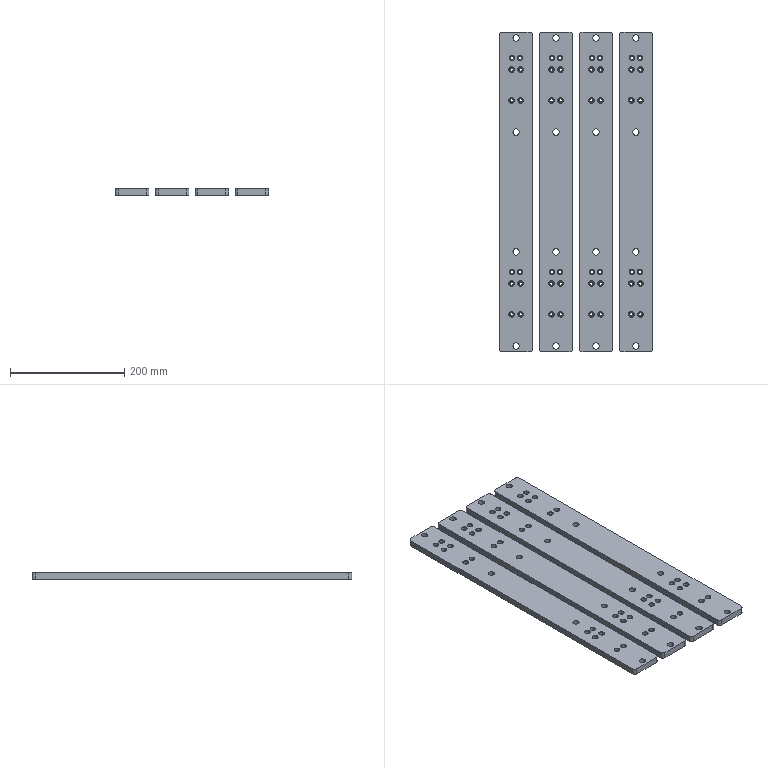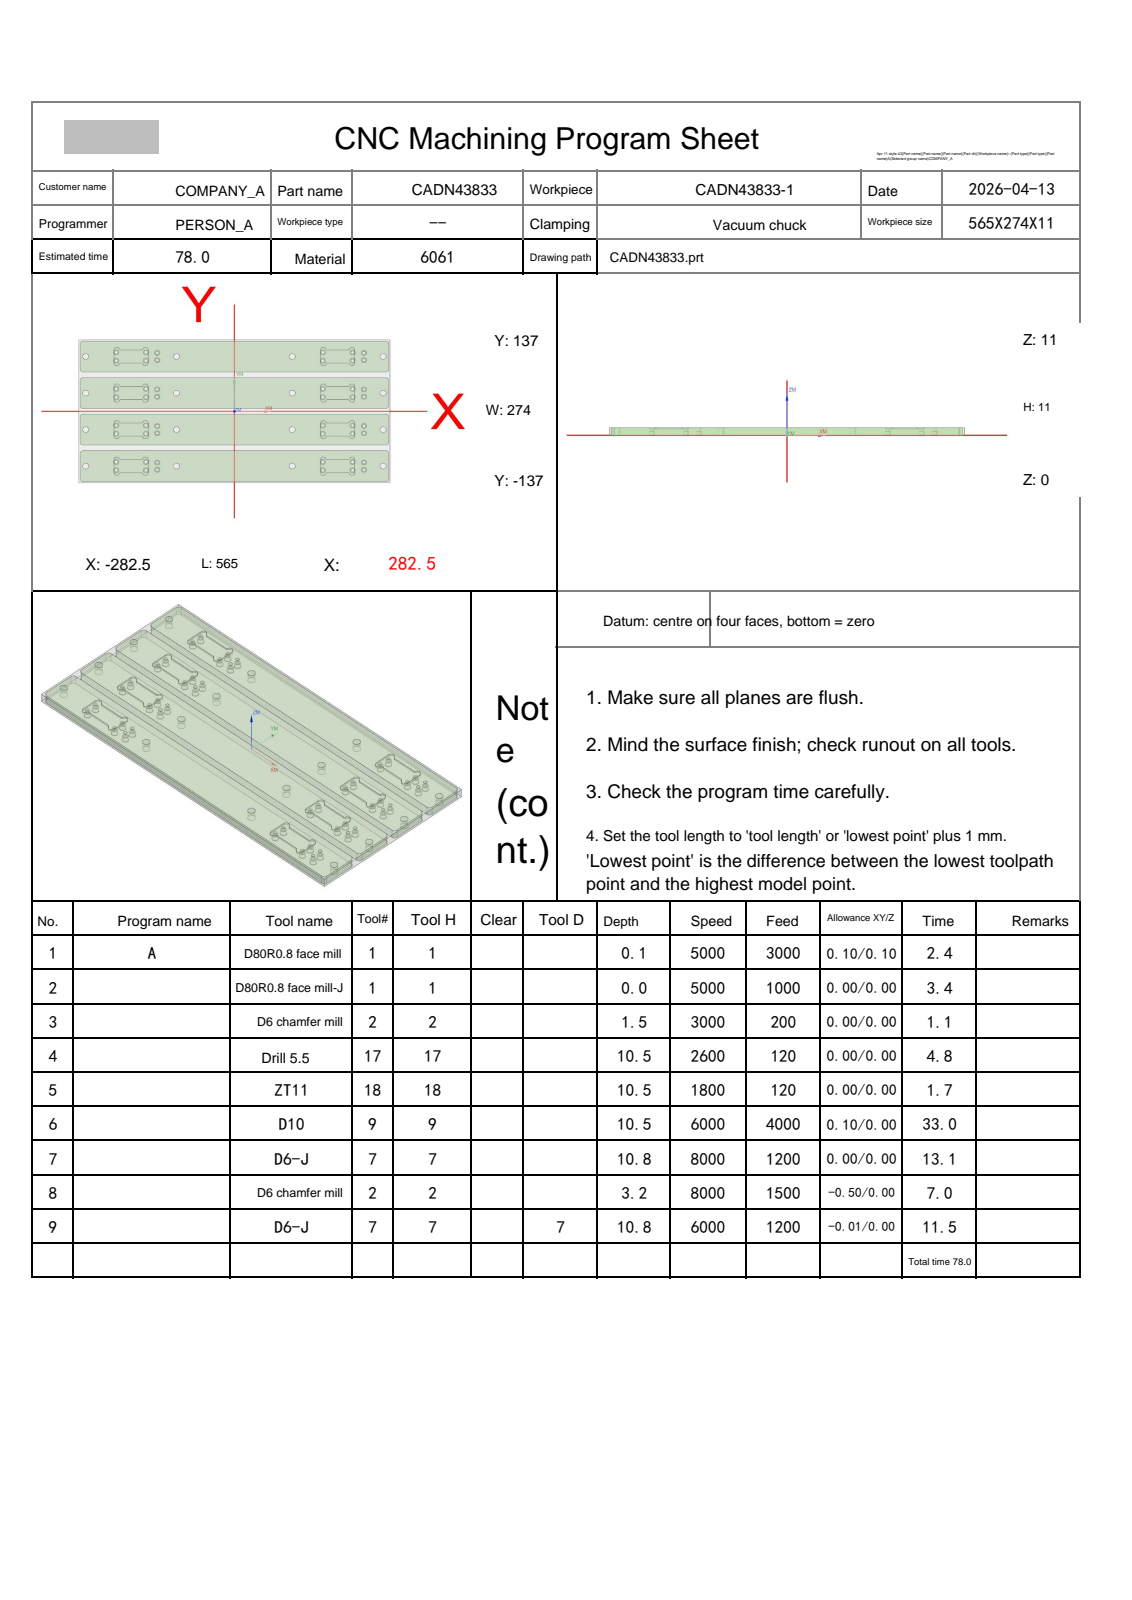NC program | NX | posted by the shop | part box 269 x 560 x 11 mm
Lines 1 to 1918 of 6644, first 1868 of 1916 lines:
%
O0001
(Machine time: 79.36 MIN)
(===Total Tool:6===)
(T1=D80R0.8 face mill D=80.  R=0.8  D-  H01 Z=11.   )
(T2=D6 chamfer mill   D=6.   R=0.   D-  H02 Z=7.8   )
(T17=drill 5.5  D=5.5  DR_a=118 D-  H17 Z=0.5   )
(T18=ZT11   D=11.  DR_a=118 D-  H18 Z=0.5   )
(T9=D10     D=10.  R=0.   D-  H09 Z=0.5   )
(T7=D6-J    D=6.   R=0.   D7  H07 Z=0.2   )
G80 G90 G17 G49 G40
G91 G28 Z0
M01
N1 T01 M06
(D80R0.8 face mill  D=80. R=0.8 H=01 ce=0.10 di=0.10)
G00 G90 G54 X-332.097 Y109.93 M03 S5000
G43 H01 Z31.
M08
Z13.55
G01 Z11.55 F3000.
X-320.097 Y110.07
X312.818 Y117.441
X312.897 Y117.442
G02 X320.097 Y110.246 I0.0 J-7.2
G01 Y80.507
Y80.493
X320.074 Y70.351
G02 X312.172 Y62.375 I-8. J.023
G01 X-312.195 Y55.103
G03 X-320.097 Y47.109 I.098 J-7.999
G01 Y10.514
Y10.486
X-320.084 Y7.204
G03 X-312.885 Y.037 I7.2 J.032
G01 X-312.805
X312.794 Y7.323
X312.873 Y7.324
G02 X320.073 Y.144 I0.0 J-7.2
G01 X320.097 Y-10.492
Y-10.508
Y-39.748
G02 X312.195 Y-47.743 I-8. J.004
G01 X-312.195 Y-55.015
G03 X-320.097 Y-63.009 I.098 J-7.999
G01 Y-102.881
G03 X-312.897 Y-110.081 I7.2 J0.0
G01 X-312.813
X320.097 Y-102.71
X332.097 Y-102.57
Z13.55
G00 X-332.097 Y109.93
Z13.1
G01 Z11.1
X-320.097 Y110.07
X312.818 Y117.441
X312.897 Y117.442
G02 X320.097 Y110.246 I0.0 J-7.2
G01 Y80.507
Y80.493
X320.074 Y70.351
G02 X312.172 Y62.375 I-8. J.023
G01 X-312.195 Y55.103
G03 X-320.097 Y47.109 I.098 J-7.999
G01 Y10.514
Y10.486
X-320.084 Y7.204
G03 X-312.885 Y.037 I7.2 J.032
G01 X-312.805
X312.794 Y7.323
X312.873 Y7.324
G02 X320.073 Y.144 I0.0 J-7.2
G01 X320.097 Y-10.492
Y-10.508
Y-39.748
G02 X312.195 Y-47.743 I-8. J.004
G01 X-312.195 Y-55.015
G03 X-320.097 Y-63.009 I.098 J-7.999
G01 Y-102.881
G03 X-312.897 Y-110.081 I7.2 J0.0
G01 X-312.813
X320.097 Y-102.71
X332.097 Y-102.57
Z13.1
G00 Z31.
G91 G28 Z0.0
M05
M09
G91 G28 Z0.0
M01
N2 T01 M06
(D80R0.8 face mill-J  D=80. R=0.8 H=01 ce=0.00 di=0.00)
G00 G90 G54 X-331.999 Y109.833 M03 S5000
G43 H01 Z31.
M08
Z13.
G01 Z11. F1000.
X-319.999 Y109.973
X312.72 Y117.35
X312.799
G02 X319.999 Y110.154 I0.0 J-7.2
G01 Y80.507
Y80.493
X319.977 Y70.307
G02 X312.075 Y62.33 I-8. J.023
G01 X-312.097 Y55.053
G03 X-319.999 Y47.059 I.098 J-7.999
G01 Y10.514
Y10.486
X-319.987 Y7.202
G03 X-312.787 Y.034 I7.2 J.032
G01 X-312.708
X312.696 Y7.326
X312.776
G02 X319.976 Y.147 I0.0 J-7.2
G01 X319.999 Y-10.493
Y-10.507
Y-39.698
G02 X312.097 Y-47.693 I-8. J.005
G01 X-312.097 Y-54.97
G03 X-319.999 Y-62.965 I.098 J-7.999
G01 Y-80.5
Y-102.794
G03 X-312.799 Y-109.989 I7.2 J.005
G01 X-312.72
X319.999 Y-102.612
X331.999 Y-102.472
Z13.
G00 Z31.
G91 G28 Z0.0
M05
M09
G91 G28 Z0.0
M01
N3 T02 M06
(D6 chamfer mill  D=6. R=0. H=02 ce=0.00 di=0.00)
G00 G90 G54 X105. Y35. M03 S3000
G43 H02 Z31.
M08
G98 G81 X105. Y35. Z9.5 R12. F200.
X160.5 Y43.
Y27.
Y-27.
Y-43.
X105. Y-35.
Y-105.
X160.5 Y-97.
Y-113.
X214.5
Y-97.
X235. Y-98.
Y-112.
X270. Y-105.
Y-35.
X235. Y-28.
Y-42.
X214.5 Y-43.
Y-27.
Y27.
Y43.
X235. Y42.
Y28.
X270. Y35.
Y105.
X235. Y112.
Y98.
X214.5 Y97.
Y113.
X160.5
Y97.
X105. Y105.
X-105.
X-140. Y112.
Y98.
X-160.5 Y97.
Y113.
X-214.5
Y97.
X-270. Y105.
Y35.
X-214.5 Y43.
Y27.
X-160.5
Y43.
X-140. Y42.
Y28.
X-105. Y35.
Y-35.
X-140. Y-42.
Y-28.
X-160.5 Y-27.
Y-43.
X-214.5
Y-27.
X-270. Y-35.
Y-105.
X-214.5 Y-97.
Y-113.
X-160.5
Y-97.
X-140. Y-98.
Y-112.
X-105. Y-105.
G80
G00 Z31.
G91 G28 Z0.0
M05
M09
G91 G28 Z0.0
M01
N4 T17 M06
(drill 5.5 D=5.5 DR_a=118 H=17)
G00 G90 G54 X-160.5 Y27. M03 S2600
G43 H17 Z31.
M08
G98 G83 X-160.5 Y27. Z.5 R12. F120. Q1.5
Y43.
X-140. Y42.
Y28.
Y-28.
X-160.5 Y-27.
Y-43.
X-140. Y-42.
Y-98.
Y-112.
X-160.5 Y-113.
Y-97.
X-214.5 Y-113.
Y-97.
Y-43.
Y-27.
Y27.
Y43.
Y97.
Y113.
X-160.5
Y97.
X-140. Y98.
Y112.
X160.5 Y113.
Y97.
Y43.
Y27.
Y-27.
Y-43.
Y-97.
Y-113.
X214.5
X235. Y-112.
Y-98.
X214.5 Y-97.
Y-43.
X235. Y-42.
Y-28.
X214.5 Y-27.
Y27.
X235. Y28.
Y42.
X214.5 Y43.
Y97.
Y113.
X235. Y112.
Y98.
G80
G00 Z31.
G91 G28 Z0.0
M05
M09
G91 G28 Z0.0
M01
N5 T18 M06
(ZT11 D=11. DR_a=118 H=18)
G00 G90 G54 X-270. Y-105. M03 S1800
G43 H18 Z31.
M08
G98 G83 X-270. Y-105. Z.5 R12. F120. Q1.5
Y-35.
Y35.
Y105.
X-105.
Y35.
Y-35.
Y-105.
X105.
Y-35.
Y35.
Y105.
X270.
Y35.
Y-35.
Y-105.
G80
G00 Z31.
G91 G28 Z0.0
M05
M09
G91 G28 Z0.0
M01
N6 T09 M06
(D10  D=10. R=0. H=09 ce=0.10 di=0.10)
G00 G90 G54 X177.82 Y-104.85 M03 S6000
G43 H09 Z31.
M08
Z11.5
M03 S6000
G01 X168.85 Z11.187 F2800.
Y-105.15 Z11.176
X187.5 Z10.525
Y-105.45
M03 S6000
X206.45 F3500.
Y-104.55
X168.55
Y-105.45
X187.5
Y-112.45
X206.792
G02 X213.45 Y-117.182 I0.0 J-7.05
G01 Y-92.818
G02 X206.792 Y-97.55 I-6.658 J2.318
G01 X168.208
G02 X161.55 Y-92.818 I0.0 J7.05
G01 Y-117.182
G02 X168.208 Y-112.45 I6.658 J-2.318
G01 X187.5
Z11.525
G00 Z12.
X177.82 Y-104.85
Z11.025
M03 S6000
G01 X168.85 Z10.712 F2800.
Y-105.15 Z10.701
X187.5 Z10.05
Y-105.45
M03 S6000
X206.45 F3500.
Y-104.55
X168.55
Y-105.45
X187.5
Y-112.45
X206.792
G02 X213.45 Y-117.182 I0.0 J-7.05
G01 Y-92.818
G02 X206.792 Y-97.55 I-6.658 J2.318
G01 X168.208
G02 X161.55 Y-92.818 I0.0 J7.05
G01 Y-117.182
G02 X168.208 Y-112.45 I6.658 J-2.318
G01 X187.5
Z11.05
G00 Z11.525
X177.82 Y-104.85
Z10.55
M03 S6000
G01 X168.85 Z10.237 F2800.
Y-105.15 Z10.226
X187.5 Z9.575
Y-105.45
M03 S6000
X206.45 F3500.
Y-104.55
X168.55
Y-105.45
X187.5
Y-112.45
X206.792
G02 X213.45 Y-117.182 I0.0 J-7.05
G01 Y-92.818
G02 X206.792 Y-97.55 I-6.658 J2.318
G01 X168.208
G02 X161.55 Y-92.818 I0.0 J7.05
G01 Y-117.182
G02 X168.208 Y-112.45 I6.658 J-2.318
G01 X187.5
Z10.575
G00 Z11.05
X177.82 Y-104.85
Z10.075
M03 S6000
G01 X168.85 Z9.762 F2800.
Y-105.15 Z9.751
X187.5 Z9.1
Y-105.45
M03 S6000
X206.45 F3500.
Y-104.55
X168.55
Y-105.45
X187.5
Y-112.45
X206.792
G02 X213.45 Y-117.182 I0.0 J-7.05
G01 Y-92.818
G02 X206.792 Y-97.55 I-6.658 J2.318
G01 X168.208
G02 X161.55 Y-92.818 I0.0 J7.05
G01 Y-117.182
G02 X168.208 Y-112.45 I6.658 J-2.318
G01 X187.5
Z10.1
G00 Z31.
X177.82 Y-34.85
Z11.5
M03 S6000
G01 X168.85 Z11.187 F2800.
Y-35.15 Z11.176
X187.5 Z10.525
Y-35.45
M03 S6000
X206.45 F3500.
Y-34.55
X168.55
Y-35.45
X187.5
Y-42.45
X206.792
G02 X213.45 Y-47.182 I0.0 J-7.05
G01 Y-22.818
G02 X206.792 Y-27.55 I-6.658 J2.318
G01 X168.208
G02 X161.55 Y-22.818 I0.0 J7.05
G01 Y-47.182
G02 X168.208 Y-42.45 I6.658 J-2.318
G01 X187.5
Z11.525
G00 Z12.
X177.82 Y-34.85
Z11.025
M03 S6000
G01 X168.85 Z10.712 F2800.
Y-35.15 Z10.701
X187.5 Z10.05
Y-35.45
M03 S6000
X206.45 F3500.
Y-34.55
X168.55
Y-35.45
X187.5
Y-42.45
X206.792
G02 X213.45 Y-47.182 I0.0 J-7.05
G01 Y-22.818
G02 X206.792 Y-27.55 I-6.658 J2.318
G01 X168.208
G02 X161.55 Y-22.818 I0.0 J7.05
G01 Y-47.182
G02 X168.208 Y-42.45 I6.658 J-2.318
G01 X187.5
Z11.05
G00 Z11.525
X177.82 Y-34.85
Z10.55
M03 S6000
G01 X168.85 Z10.237 F2800.
Y-35.15 Z10.226
X187.5 Z9.575
Y-35.45
M03 S6000
X206.45 F3500.
Y-34.55
X168.55
Y-35.45
X187.5
Y-42.45
X206.792
G02 X213.45 Y-47.182 I0.0 J-7.05
G01 Y-22.818
G02 X206.792 Y-27.55 I-6.658 J2.318
G01 X168.208
G02 X161.55 Y-22.818 I0.0 J7.05
G01 Y-47.182
G02 X168.208 Y-42.45 I6.658 J-2.318
G01 X187.5
Z10.575
G00 Z11.05
X177.82 Y-34.85
Z10.075
M03 S6000
G01 X168.85 Z9.762 F2800.
Y-35.15 Z9.751
X187.5 Z9.1
Y-35.45
M03 S6000
X206.45 F3500.
Y-34.55
X168.55
Y-35.45
X187.5
Y-42.45
X206.792
G02 X213.45 Y-47.182 I0.0 J-7.05
G01 Y-22.818
G02 X206.792 Y-27.55 I-6.658 J2.318
G01 X168.208
G02 X161.55 Y-22.818 I0.0 J7.05
G01 Y-47.182
G02 X168.208 Y-42.45 I6.658 J-2.318
G01 X187.5
Z10.1
G00 Z31.
X177.82 Y35.15
Z11.5
M03 S6000
G01 X168.85 Z11.187 F2800.
Y34.85 Z11.176
X187.5 Z10.525
Y34.55
M03 S6000
X206.45 F3500.
Y35.45
X168.55
Y34.55
X187.5
Y27.55
X206.792
G02 X213.45 Y22.818 I0.0 J-7.05
G01 Y47.182
G02 X206.792 Y42.45 I-6.658 J2.318
G01 X168.208
G02 X161.55 Y47.182 I0.0 J7.05
G01 Y22.818
G02 X168.208 Y27.55 I6.658 J-2.318
G01 X187.5
Z11.525
G00 Z12.
X177.82 Y35.15
Z11.025
M03 S6000
G01 X168.85 Z10.712 F2800.
Y34.85 Z10.701
X187.5 Z10.05
Y34.55
M03 S6000
X206.45 F3500.
Y35.45
X168.55
Y34.55
X187.5
Y27.55
X206.792
G02 X213.45 Y22.818 I0.0 J-7.05
G01 Y47.182
G02 X206.792 Y42.45 I-6.658 J2.318
G01 X168.208
G02 X161.55 Y47.182 I0.0 J7.05
G01 Y22.818
G02 X168.208 Y27.55 I6.658 J-2.318
G01 X187.5
Z11.05
G00 Z11.525
X177.82 Y35.15
Z10.55
M03 S6000
G01 X168.85 Z10.237 F2800.
Y34.85 Z10.226
X187.5 Z9.575
Y34.55
M03 S6000
X206.45 F3500.
Y35.45
X168.55
Y34.55
X187.5
Y27.55
X206.792
G02 X213.45 Y22.818 I0.0 J-7.05
G01 Y47.182
G02 X206.792 Y42.45 I-6.658 J2.318
G01 X168.208
G02 X161.55 Y47.182 I0.0 J7.05
G01 Y22.818
G02 X168.208 Y27.55 I6.658 J-2.318
G01 X187.5
Z10.575
G00 Z11.05
X177.82 Y35.15
Z10.075
M03 S6000
G01 X168.85 Z9.762 F2800.
Y34.85 Z9.751
X187.5 Z9.1
Y34.55
M03 S6000
X206.45 F3500.
Y35.45
X168.55
Y34.55
X187.5
Y27.55
X206.792
G02 X213.45 Y22.818 I0.0 J-7.05
G01 Y47.182
G02 X206.792 Y42.45 I-6.658 J2.318
G01 X168.208
G02 X161.55 Y47.182 I0.0 J7.05
G01 Y22.818
G02 X168.208 Y27.55 I6.658 J-2.318
G01 X187.5
Z10.1
G00 Z31.
X197.18 Y104.85
Z11.5
M03 S6000
G01 X206.15 Z11.187 F2800.
Y105.15 Z11.176
X187.5 Z10.525
Y105.45
M03 S6000
X168.55 F3500.
Y104.55
X206.45
Y105.45
X187.5
Y112.45
X168.208
G02 X161.55 Y117.182 I0.0 J7.05
G01 Y92.818
G02 X168.208 Y97.55 I6.658 J-2.318
G01 X206.792
G02 X213.45 Y92.818 I0.0 J-7.05
G01 Y117.182
G02 X206.792 Y112.45 I-6.658 J2.318
G01 X187.5
Z11.525
G00 Z12.
X197.18 Y104.85
Z11.025
M03 S6000
G01 X206.15 Z10.712 F2800.
Y105.15 Z10.701
X187.5 Z10.05
Y105.45
M03 S6000
X168.55 F3500.
Y104.55
X206.45
Y105.45
X187.5
Y112.45
X168.208
G02 X161.55 Y117.182 I0.0 J7.05
G01 Y92.818
G02 X168.208 Y97.55 I6.658 J-2.318
G01 X206.792
G02 X213.45 Y92.818 I0.0 J-7.05
G01 Y117.182
G02 X206.792 Y112.45 I-6.658 J2.318
G01 X187.5
Z11.05
G00 Z11.525
X197.18 Y104.85
Z10.55
M03 S6000
G01 X206.15 Z10.237 F2800.
Y105.15 Z10.226
X187.5 Z9.575
Y105.45
M03 S6000
X168.55 F3500.
Y104.55
X206.45
Y105.45
X187.5
Y112.45
X168.208
G02 X161.55 Y117.182 I0.0 J7.05
G01 Y92.818
G02 X168.208 Y97.55 I6.658 J-2.318
G01 X206.792
G02 X213.45 Y92.818 I0.0 J-7.05
G01 Y117.182
G02 X206.792 Y112.45 I-6.658 J2.318
G01 X187.5
Z10.575
G00 Z11.05
X197.18 Y104.85
Z10.075
M03 S6000
G01 X206.15 Z9.762 F2800.
Y105.15 Z9.751
X187.5 Z9.1
Y105.45
M03 S6000
X168.55 F3500.
Y104.55
X206.45
Y105.45
X187.5
Y112.45
X168.208
G02 X161.55 Y117.182 I0.0 J7.05
G01 Y92.818
G02 X168.208 Y97.55 I6.658 J-2.318
G01 X206.792
G02 X213.45 Y92.818 I0.0 J-7.05
G01 Y117.182
G02 X206.792 Y112.45 I-6.658 J2.318
G01 X187.5
Z10.1
G00 Z31.
X-177.82 Y104.85
Z11.5
M03 S6000
G01 X-168.85 Z11.187 F2800.
Y105.15 Z11.176
X-187.5 Z10.525
Y105.45
M03 S6000
X-206.45 F3500.
Y104.55
X-168.55
Y105.45
X-187.5
Y112.45
X-206.792
G02 X-213.45 Y117.182 I0.0 J7.05
G01 Y92.818
G02 X-206.792 Y97.55 I6.658 J-2.318
G01 X-168.208
G02 X-161.55 Y92.818 I0.0 J-7.05
G01 Y117.182
G02 X-168.208 Y112.45 I-6.658 J2.318
G01 X-187.5
Z11.525
G00 Z12.
X-177.82 Y104.85
Z11.025
M03 S6000
G01 X-168.85 Z10.712 F2800.
Y105.15 Z10.701
X-187.5 Z10.05
Y105.45
M03 S6000
X-206.45 F3500.
Y104.55
X-168.55
Y105.45
X-187.5
Y112.45
X-206.792
G02 X-213.45 Y117.182 I0.0 J7.05
G01 Y92.818
G02 X-206.792 Y97.55 I6.658 J-2.318
G01 X-168.208
G02 X-161.55 Y92.818 I0.0 J-7.05
G01 Y117.182
G02 X-168.208 Y112.45 I-6.658 J2.318
G01 X-187.5
Z11.05
G00 Z11.525
X-177.82 Y104.85
Z10.55
M03 S6000
G01 X-168.85 Z10.237 F2800.
Y105.15 Z10.226
X-187.5 Z9.575
Y105.45
M03 S6000
X-206.45 F3500.
Y104.55
X-168.55
Y105.45
X-187.5
Y112.45
X-206.792
G02 X-213.45 Y117.182 I0.0 J7.05
G01 Y92.818
G02 X-206.792 Y97.55 I6.658 J-2.318
G01 X-168.208
G02 X-161.55 Y92.818 I0.0 J-7.05
G01 Y117.182
G02 X-168.208 Y112.45 I-6.658 J2.318
G01 X-187.5
Z10.575
G00 Z11.05
X-177.82 Y104.85
Z10.075
M03 S6000
G01 X-168.85 Z9.762 F2800.
Y105.15 Z9.751
X-187.5 Z9.1
Y105.45
M03 S6000
X-206.45 F3500.
Y104.55
X-168.55
Y105.45
X-187.5
Y112.45
X-206.792
G02 X-213.45 Y117.182 I0.0 J7.05
G01 Y92.818
G02 X-206.792 Y97.55 I6.658 J-2.318
G01 X-168.208
G02 X-161.55 Y92.818 I0.0 J-7.05
G01 Y117.182
G02 X-161.664 Y116.878 I-6.658 J2.318
X-168.208 Y112.45 I-6.544 J2.622
G01 X-187.5
Z10.1
G00 Z31.
X-177.82 Y34.85
Z11.5
M03 S6000
G01 X-168.85 Z11.187 F2800.
Y35.15 Z11.176
X-187.5 Z10.525
Y35.45
M03 S6000
X-206.45 F3500.
Y34.55
X-168.55
Y35.45
X-187.5
Y42.45
X-206.792
G02 X-213.45 Y47.182 I0.0 J7.05
G01 Y22.818
G02 X-206.792 Y27.55 I6.658 J-2.318
G01 X-168.208
G02 X-161.56 Y22.847 I0.0 J-7.05
G01 X-161.55 Y22.836
Y47.166
X-161.56 Y47.153
G02 X-168.208 Y42.45 I-6.648 J2.347
G01 X-187.5
Z11.525
G00 Z12.
X-177.82 Y34.85
Z11.025
M03 S6000
G01 X-168.85 Z10.712 F2800.
Y35.15 Z10.701
X-187.5 Z10.05
Y35.45
M03 S6000
X-206.45 F3500.
Y34.55
X-168.55
Y35.45
X-187.5
Y42.45
X-206.792
G02 X-213.45 Y47.182 I0.0 J7.05
G01 Y22.818
G02 X-206.792 Y27.55 I6.658 J-2.318
G01 X-168.208
G02 X-161.56 Y22.847 I0.0 J-7.05
G01 X-161.55 Y22.836
Y47.166
X-161.56 Y47.153
G02 X-168.208 Y42.45 I-6.648 J2.347
G01 X-187.5
Z11.05
G00 Z11.525
X-177.82 Y34.85
Z10.55
M03 S6000
G01 X-168.85 Z10.237 F2800.
Y35.15 Z10.226
X-187.5 Z9.575
Y35.45
M03 S6000
X-206.45 F3500.
Y34.55
X-168.55
Y35.45
X-187.5
Y42.45
X-206.792
G02 X-213.45 Y47.182 I0.0 J7.05
G01 Y22.818
G02 X-206.792 Y27.55 I6.658 J-2.318
G01 X-168.208
G02 X-161.56 Y22.847 I0.0 J-7.05
G01 X-161.55 Y22.836
Y47.166
X-161.56 Y47.153
G02 X-168.208 Y42.45 I-6.648 J2.347
G01 X-187.5
Z10.575
G00 Z11.05
X-177.82 Y34.85
Z10.075
M03 S6000
G01 X-168.85 Z9.762 F2800.
Y35.15 Z9.751
X-187.5 Z9.1
Y35.45
M03 S6000
X-206.45 F3500.
Y34.55
X-168.55
Y35.45
X-187.5
Y42.45
X-206.792
G02 X-213.45 Y47.182 I0.0 J7.05
G01 Y22.818
G02 X-206.792 Y27.55 I6.658 J-2.318
G01 X-168.208
G02 X-161.56 Y22.847 I0.0 J-7.05
G01 X-161.55 Y22.836
Y47.166
X-161.56 Y47.153
G02 X-168.208 Y42.45 I-6.648 J2.347
G01 X-187.5
Z10.1
G00 Z31.
X-177.82 Y-35.15
Z11.5
M03 S6000
G01 X-168.85 Z11.187 F2800.
Y-34.85 Z11.176
X-187.5 Z10.525
Y-34.55
M03 S6000
X-206.45 F3500.
Y-35.45
X-168.55
Y-34.55
X-187.5
Y-27.55
X-206.792
G02 X-213.45 Y-22.818 I0.0 J7.05
G01 Y-47.182
G02 X-206.792 Y-42.45 I6.658 J-2.318
G01 X-168.208
G02 X-161.55 Y-47.182 I0.0 J-7.05
G01 Y-22.818
G02 X-168.208 Y-27.55 I-6.658 J2.318
G01 X-187.5
Z11.525
G00 Z12.
X-177.82 Y-35.15
Z11.025
M03 S6000
G01 X-168.85 Z10.712 F2800.
Y-34.85 Z10.701
X-187.5 Z10.05
Y-34.55
M03 S6000
X-206.45 F3500.
Y-35.45
X-168.55
Y-34.55
X-187.5
Y-27.55
X-206.792
G02 X-213.45 Y-22.818 I0.0 J7.05
G01 Y-47.182
G02 X-206.792 Y-42.45 I6.658 J-2.318
G01 X-168.208
G02 X-161.55 Y-47.182 I0.0 J-7.05
G01 Y-22.818
G02 X-168.208 Y-27.55 I-6.658 J2.318
G01 X-187.5
Z11.05
G00 Z11.525
X-177.82 Y-35.15
Z10.55
M03 S6000
G01 X-168.85 Z10.237 F2800.
Y-34.85 Z10.226
X-187.5 Z9.575
Y-34.55
M03 S6000
X-206.45 F3500.
Y-35.45
X-168.55
Y-34.55
X-187.5
Y-27.55
X-206.792
G02 X-213.45 Y-22.818 I0.0 J7.05
G01 Y-47.144
Y-47.182
G02 X-206.792 Y-42.45 I6.658 J-2.318
G01 X-168.208
G02 X-161.55 Y-47.182 I0.0 J-7.05
G01 Y-22.818
G02 X-168.208 Y-27.55 I-6.658 J2.318
G01 X-187.5
Z10.575
G00 Z11.05
X-177.82 Y-35.15
Z10.075
M03 S6000
G01 X-168.85 Z9.762 F2800.
Y-34.85 Z9.751
X-187.5 Z9.1
Y-34.55
M03 S6000
X-206.45 F3500.
Y-35.45
X-168.55
Y-34.55
X-187.5
Y-27.55
X-206.792
G02 X-213.45 Y-22.818 I0.0 J7.05
G01 Y-47.144
Y-47.182
G02 X-206.792 Y-42.45 I6.658 J-2.318
G01 X-168.208
G02 X-161.55 Y-47.182 I0.0 J-7.05
G01 Y-22.818
G02 X-168.208 Y-27.55 I-6.658 J2.318
G01 X-187.5
Z10.1
G00 Z31.
X-197.18 Y-104.85
Z11.5
M03 S6000
G01 X-206.15 Z11.187 F2800.
Y-105.15 Z11.176
X-187.5 Z10.525
Y-105.45
M03 S6000
X-168.55 F3500.
Y-104.55
X-206.45
Y-105.45
X-187.5
Y-112.45
X-168.208
G02 X-161.55 Y-117.182 I0.0 J-7.05
G01 Y-92.818
G02 X-168.208 Y-97.55 I-6.658 J2.318
G01 X-206.792
G02 X-213.45 Y-92.818 I0.0 J7.05
G01 Y-117.182
G02 X-206.792 Y-112.45 I6.658 J-2.318
G01 X-187.5
Z11.525
G00 Z12.
X-197.18 Y-104.85
Z11.025
M03 S6000
G01 X-206.15 Z10.712 F2800.
Y-105.15 Z10.701
X-187.5 Z10.05
Y-105.45
M03 S6000
X-168.55 F3500.
Y-104.55
X-206.45
Y-105.45
X-187.5
Y-112.45
X-168.208
G02 X-161.55 Y-117.182 I0.0 J-7.05
G01 Y-92.818
G02 X-168.208 Y-97.55 I-6.658 J2.318
G01 X-206.792
G02 X-213.45 Y-92.818 I0.0 J7.05
G01 Y-117.182
G02 X-206.792 Y-112.45 I6.658 J-2.318
G01 X-187.5
Z11.05
G00 Z11.525
X-197.18 Y-104.85
Z10.55
M03 S6000
G01 X-206.15 Z10.237 F2800.
Y-105.15 Z10.226
X-187.5 Z9.575
Y-105.45
M03 S6000
X-168.55 F3500.
Y-104.55
X-206.45
Y-105.45
X-187.5
Y-112.45
X-168.208
G02 X-161.55 Y-117.182 I0.0 J-7.05
G01 Y-92.818
G02 X-161.654 Y-93.098 I-6.658 J2.318
X-168.208 Y-97.55 I-6.554 J2.598
G01 X-206.792
G02 X-213.45 Y-92.818 I0.0 J7.05
G01 Y-117.182
G02 X-206.792 Y-112.45 I6.658 J-2.318
G01 X-187.5
Z10.575
G00 Z11.05
X-197.18 Y-104.85
Z10.075
M03 S6000
G01 X-206.15 Z9.762 F2800.
Y-105.15 Z9.751
X-187.5 Z9.1
Y-105.45
M03 S6000
X-168.55 F3500.
Y-104.55
X-206.45
Y-105.45
X-187.5
Y-112.45
X-168.208
G02 X-161.55 Y-117.182 I0.0 J-7.05
G01 Y-92.818
X-161.568 Y-92.869
G02 X-168.208 Y-97.55 I-6.64 J2.369
G01 X-206.792
G02 X-213.45 Y-92.818 I0.0 J7.05
G01 Y-117.182
G02 X-206.792 Y-112.45 I6.658 J-2.318
G01 X-187.5
Z10.1
G00 Z31.
G00 G90 X0.0 Y139.6 M03 S6000
Z31.
Z11.5
G01 X275. Z11.396 F4000.
G02 X285.1 Y129.5 Z11.39 I0.0 J-10.1
G01 Y80.5 Z11.371
G02 X275. Y70.4 Z11.365 I-10.1 J0.0
G01 X-275. Z11.157
G02 X-285.1 Y80.5 Z11.151 I0.0 J10.1
G01 Y129.5 Z11.132
G02 X-275. Y139.6 Z11.126 I10.1 J0.0
G01 X275. Z10.917
G02 X285.1 Y129.5 Z10.911 I0.0 J-10.1
G01 Y80.5 Z10.893
G02 X275. Y70.4 Z10.887 I-10.1 J0.0
G01 X-275. Z10.678
G02 X-285.1 Y80.5 Z10.672 I0.0 J10.1
G01 Y129.5 Z10.654
G02 X-275. Y139.6 Z10.648 I10.1 J0.0
G01 X275. Z10.439
G02 X285.1 Y129.5 Z10.433 I0.0 J-10.1
G01 Y80.5 Z10.415
G02 X275. Y70.4 Z10.409 I-10.1 J0.0
G01 X-275. Z10.2
G02 X-285.1 Y80.5 Z10.194 I0.0 J10.1
G01 Y129.5 Z10.175
G02 X-275. Y139.6 Z10.169 I10.1 J0.0
G01 X275. Z9.961
G02 X285.1 Y129.5 Z9.955 I0.0 J-10.1
G01 Y80.5 Z9.936
G02 X275. Y70.4 Z9.93 I-10.1 J0.0
G01 X-275. Z9.722
G02 X-285.1 Y80.5 Z9.716 I0.0 J10.1
G01 Y129.5 Z9.697
G02 X-275. Y139.6 Z9.691 I10.1 J0.0
G01 X275. Z9.483
G02 X285.1 Y129.5 Z9.477 I0.0 J-10.1
G01 Y80.5 Z9.458
G02 X275. Y70.4 Z9.452 I-10.1 J0.0
G01 X-275. Z9.244
G02 X-285.1 Y80.5 Z9.238 I0.0 J10.1
G01 Y129.5 Z9.219
G02 X-275. Y139.6 Z9.213 I10.1 J0.0
G01 X275. Z9.004
G02 X285.1 Y129.5 Z8.998 I0.0 J-10.1
G01 Y80.5 Z8.98
G02 X275. Y70.4 Z8.974 I-10.1 J0.0
G01 X-275. Z8.765
G02 X-285.1 Y80.5 Z8.759 I0.0 J10.1
G01 Y129.5 Z8.741
G02 X-275. Y139.6 Z8.735 I10.1 J0.0
G01 X275. Z8.526
G02 X285.1 Y129.5 Z8.52 I0.0 J-10.1
G01 Y80.5 Z8.502
G02 X275. Y70.4 Z8.496 I-10.1 J0.0
G01 X-275. Z8.287
G02 X-285.1 Y80.5 Z8.281 I0.0 J10.1
G01 Y129.5 Z8.262
G02 X-275. Y139.6 Z8.256 I10.1 J0.0
G01 X275. Z8.048
G02 X285.1 Y129.5 Z8.042 I0.0 J-10.1
G01 Y80.5 Z8.023
G02 X275. Y70.4 Z8.017 I-10.1 J0.0
G01 X-275. Z7.809
G02 X-285.1 Y80.5 Z7.803 I0.0 J10.1
G01 Y129.5 Z7.784
G02 X-275. Y139.6 Z7.778 I10.1 J0.0
G01 X275. Z7.57
G02 X285.1 Y129.5 Z7.564 I0.0 J-10.1
G01 Y80.5 Z7.545
G02 X275. Y70.4 Z7.539 I-10.1 J0.0
G01 X-275. Z7.331
G02 X-285.1 Y80.5 Z7.325 I0.0 J10.1
G01 Y129.5 Z7.306
G02 X-275. Y139.6 Z7.3 I10.1 J0.0
G01 X275. Z7.091
G02 X285.1 Y129.5 Z7.085 I0.0 J-10.1
G01 Y80.5 Z7.067
G02 X275. Y70.4 Z7.061 I-10.1 J0.0
G01 X-275. Z6.852
G02 X-285.1 Y80.5 Z6.846 I0.0 J10.1
G01 Y129.5 Z6.828
G02 X-275. Y139.6 Z6.822 I10.1 J0.0
G01 X275. Z6.613
G02 X285.1 Y129.5 Z6.607 I0.0 J-10.1
G01 Y80.5 Z6.589
G02 X275. Y70.4 Z6.583 I-10.1 J0.0
G01 X-275. Z6.374
G02 X-285.1 Y80.5 Z6.368 I0.0 J10.1
G01 Y129.5 Z6.349
G02 X-275. Y139.6 Z6.343 I10.1 J0.0
G01 X275. Z6.135
G02 X285.1 Y129.5 Z6.129 I0.0 J-10.1
G01 Y80.5 Z6.11
G02 X275. Y70.4 Z6.104 I-10.1 J0.0
G01 X-275. Z5.896
G02 X-285.1 Y80.5 Z5.89 I0.0 J10.1
G01 Y129.5 Z5.871
G02 X-275. Y139.6 Z5.865 I10.1 J0.0
G01 X275. Z5.657
G02 X285.1 Y129.5 Z5.651 I0.0 J-10.1
G01 Y80.5 Z5.632
G02 X275. Y70.4 Z5.626 I-10.1 J0.0
G01 X-275. Z5.417
G02 X-285.1 Y80.5 Z5.411 I0.0 J10.1
G01 Y129.5 Z5.393
G02 X-275. Y139.6 Z5.387 I10.1 J0.0
G01 X275. Z5.178
G02 X285.1 Y129.5 Z5.172 I0.0 J-10.1
G01 Y80.5 Z5.154
G02 X275. Y70.4 Z5.148 I-10.1 J0.0
G01 X-275. Z4.939
G02 X-285.1 Y80.5 Z4.933 I0.0 J10.1
G01 Y129.5 Z4.915
G02 X-275. Y139.6 Z4.909 I10.1 J0.0
G01 X275. Z4.7
G02 X285.1 Y129.5 Z4.694 I0.0 J-10.1
G01 Y80.5 Z4.675
G02 X275. Y70.4 Z4.669 I-10.1 J0.0
G01 X-275. Z4.461
G02 X-285.1 Y80.5 Z4.455 I0.0 J10.1
G01 Y129.5 Z4.436
G02 X-275. Y139.6 Z4.43 I10.1 J0.0
G01 X275. Z4.222
G02 X285.1 Y129.5 Z4.216 I0.0 J-10.1
G01 Y80.5 Z4.197
G02 X275. Y70.4 Z4.191 I-10.1 J0.0
G01 X-275. Z3.983
G02 X-285.1 Y80.5 Z3.977 I0.0 J10.1
G01 Y129.5 Z3.958
G02 X-275. Y139.6 Z3.952 I10.1 J0.0
G01 X275. Z3.744
G02 X285.1 Y129.5 Z3.738 I0.0 J-10.1
G01 Y80.5 Z3.719
G02 X275. Y70.4 Z3.713 I-10.1 J0.0
G01 X-275. Z3.504
G02 X-285.1 Y80.5 Z3.498 I0.0 J10.1
G01 Y129.5 Z3.48
G02 X-275. Y139.6 Z3.474 I10.1 J0.0
G01 X275. Z3.265
G02 X285.1 Y129.5 Z3.259 I0.0 J-10.1
G01 Y80.5 Z3.241
G02 X275. Y70.4 Z3.235 I-10.1 J0.0
G01 X-275. Z3.026
G02 X-285.1 Y80.5 Z3.02 I0.0 J10.1
G01 Y129.5 Z3.002
G02 X-275. Y139.6 Z2.996 I10.1 J0.0
G01 X275. Z2.787
G02 X285.1 Y129.5 Z2.781 I0.0 J-10.1
G01 Y80.5 Z2.762
G02 X275. Y70.4 Z2.756 I-10.1 J0.0
G01 X-275. Z2.548
G02 X-285.1 Y80.5 Z2.542 I0.0 J10.1
G01 Y129.5 Z2.523
G02 X-275. Y139.6 Z2.517 I10.1 J0.0
G01 X275. Z2.309
G02 X285.1 Y129.5 Z2.303 I0.0 J-10.1
G01 Y80.5 Z2.284
G02 X275. Y70.4 Z2.278 I-10.1 J0.0
G01 X-275. Z2.07
G02 X-285.1 Y80.5 Z2.064 I0.0 J10.1
G01 Y129.5 Z2.045
G02 X-275. Y139.6 Z2.039 I10.1 J0.0
G01 X275. Z1.831
G02 X285.1 Y129.5 Z1.825 I0.0 J-10.1
G01 Y80.5 Z1.806
G02 X275. Y70.4 Z1.8 I-10.1 J0.0
G01 X-275. Z1.591
G02 X-285.1 Y80.5 Z1.585 I0.0 J10.1
G01 Y129.5 Z1.567
G02 X-275. Y139.6 Z1.561 I10.1 J0.0
G01 X275. Z1.352
G02 X285.1 Y129.5 Z1.346 I0.0 J-10.1
G01 Y80.5 Z1.328
G02 X275. Y70.4 Z1.322 I-10.1 J0.0
G01 X-275. Z1.113
G02 X-285.1 Y80.5 Z1.107 I0.0 J10.1
G01 Y129.5 Z1.089
G02 X-275. Y139.6 Z1.083 I10.1 J0.0
G01 X275. Z.874
G02 X285.1 Y129.5 Z.868 I0.0 J-10.1
G01 Y80.5 Z.849
G02 X275. Y70.4 Z.843 I-10.1 J0.0
G01 X-275. Z.635
G02 X-285.1 Y80.5 Z.629 I0.0 J10.1
G01 Y129.5 Z.61
G02 X-275. Y139.6 Z.604 I10.1 J0.0
G01 X0.0 Z.5
X275.
G02 X285.1 Y129.5 I0.0 J-10.1
G01 Y80.5
G02 X275. Y70.4 I-10.1 J0.0
G01 X-275.
G02 X-285.1 Y80.5 I0.0 J10.1
G01 Y129.5
G02 X-275. Y139.6 I10.1 J0.0
G01 X0.0
X.5
Z1.5
G00 Z31.
X0.0 Y69.6
Z11.5
G01 X275. Z11.396
G02 X285.1 Y59.5 Z11.39 I0.0 J-10.1
G01 Y10.5 Z11.371
G02 X275. Y.4 Z11.365 I-10.1 J0.0
G01 X-275. Z11.157
G02 X-285.1 Y10.5 Z11.151 I0.0 J10.1
G01 Y59.5 Z11.132
G02 X-275. Y69.6 Z11.126 I10.1 J0.0
G01 X275. Z10.917
G02 X285.1 Y59.5 Z10.911 I0.0 J-10.1
G01 Y10.5 Z10.893
G02 X275. Y.4 Z10.887 I-10.1 J0.0
G01 X-275. Z10.678
G02 X-285.1 Y10.5 Z10.672 I0.0 J10.1
G01 Y59.5 Z10.654
G02 X-275. Y69.6 Z10.648 I10.1 J0.0
G01 X275. Z10.439
G02 X285.1 Y59.5 Z10.433 I0.0 J-10.1
G01 Y10.5 Z10.415
G02 X275. Y.4 Z10.409 I-10.1 J0.0
G01 X-275. Z10.2
G02 X-285.1 Y10.5 Z10.194 I0.0 J10.1
G01 Y59.5 Z10.175
G02 X-275. Y69.6 Z10.169 I10.1 J0.0
G01 X275. Z9.961
G02 X285.1 Y59.5 Z9.955 I0.0 J-10.1
G01 Y10.5 Z9.936
G02 X275. Y.4 Z9.93 I-10.1 J0.0
G01 X-275. Z9.722
G02 X-285.1 Y10.5 Z9.716 I0.0 J10.1
G01 Y59.5 Z9.697
G02 X-275. Y69.6 Z9.691 I10.1 J0.0
G01 X275. Z9.483
G02 X285.1 Y59.5 Z9.477 I0.0 J-10.1
G01 Y10.5 Z9.458
G02 X275. Y.4 Z9.452 I-10.1 J0.0
G01 X-275. Z9.244
G02 X-285.1 Y10.5 Z9.238 I0.0 J10.1
G01 Y59.5 Z9.219
G02 X-275. Y69.6 Z9.213 I10.1 J0.0
G01 X275. Z9.004
G02 X285.1 Y59.5 Z8.998 I0.0 J-10.1
G01 Y10.5 Z8.98
G02 X275. Y.4 Z8.974 I-10.1 J0.0
G01 X-275. Z8.765
G02 X-285.1 Y10.5 Z8.759 I0.0 J10.1
G01 Y59.5 Z8.741
G02 X-275. Y69.6 Z8.735 I10.1 J0.0
G01 X275. Z8.526
G02 X285.1 Y59.5 Z8.52 I0.0 J-10.1
G01 Y10.5 Z8.502
G02 X275. Y.4 Z8.496 I-10.1 J0.0
G01 X-275. Z8.287
G02 X-285.1 Y10.5 Z8.281 I0.0 J10.1
G01 Y59.5 Z8.262
G02 X-275. Y69.6 Z8.256 I10.1 J0.0
G01 X275. Z8.048
G02 X285.1 Y59.5 Z8.042 I0.0 J-10.1
G01 Y10.5 Z8.023
G02 X275. Y.4 Z8.017 I-10.1 J0.0
G01 X-275. Z7.809
G02 X-285.1 Y10.5 Z7.803 I0.0 J10.1
G01 Y59.5 Z7.784
G02 X-275. Y69.6 Z7.778 I10.1 J0.0
G01 X275. Z7.57
G02 X285.1 Y59.5 Z7.564 I0.0 J-10.1
G01 Y10.5 Z7.545
G02 X275. Y.4 Z7.539 I-10.1 J0.0
G01 X-275. Z7.331
G02 X-285.1 Y10.5 Z7.325 I0.0 J10.1
G01 Y59.5 Z7.306
G02 X-275. Y69.6 Z7.3 I10.1 J0.0
G01 X275. Z7.091
G02 X285.1 Y59.5 Z7.085 I0.0 J-10.1
G01 Y10.5 Z7.067
G02 X275. Y.4 Z7.061 I-10.1 J0.0
G01 X-275. Z6.852
G02 X-285.1 Y10.5 Z6.846 I0.0 J10.1
G01 Y59.5 Z6.828
G02 X-275. Y69.6 Z6.822 I10.1 J0.0
G01 X275. Z6.613
G02 X285.1 Y59.5 Z6.607 I0.0 J-10.1
G01 Y10.5 Z6.589
G02 X275. Y.4 Z6.583 I-10.1 J0.0
G01 X-275. Z6.374
G02 X-285.1 Y10.5 Z6.368 I0.0 J10.1
G01 Y59.5 Z6.349
G02 X-275. Y69.6 Z6.343 I10.1 J0.0
G01 X275. Z6.135
G02 X285.1 Y59.5 Z6.129 I0.0 J-10.1
G01 Y10.5 Z6.11
G02 X275. Y.4 Z6.104 I-10.1 J0.0
G01 X-275. Z5.896
G02 X-285.1 Y10.5 Z5.89 I0.0 J10.1
G01 Y59.5 Z5.871
G02 X-275. Y69.6 Z5.865 I10.1 J0.0
G01 X275. Z5.657
G02 X285.1 Y59.5 Z5.651 I0.0 J-10.1
G01 Y10.5 Z5.632
G02 X275. Y.4 Z5.626 I-10.1 J0.0
G01 X-275. Z5.417
G02 X-285.1 Y10.5 Z5.411 I0.0 J10.1
G01 Y59.5 Z5.393
G02 X-275. Y69.6 Z5.387 I10.1 J0.0
G01 X275. Z5.178
G02 X285.1 Y59.5 Z5.172 I0.0 J-10.1
G01 Y10.5 Z5.154
G02 X275. Y.4 Z5.148 I-10.1 J0.0
G01 X-275. Z4.939
G02 X-285.1 Y10.5 Z4.933 I0.0 J10.1
G01 Y59.5 Z4.915
G02 X-275. Y69.6 Z4.909 I10.1 J0.0
G01 X275. Z4.7
G02 X285.1 Y59.5 Z4.694 I0.0 J-10.1
G01 Y10.5 Z4.675
G02 X275. Y.4 Z4.669 I-10.1 J0.0
G01 X-275. Z4.461
G02 X-285.1 Y10.5 Z4.455 I0.0 J10.1
G01 Y59.5 Z4.436
G02 X-275. Y69.6 Z4.43 I10.1 J0.0
G01 X275. Z4.222
G02 X285.1 Y59.5 Z4.216 I0.0 J-10.1
G01 Y10.5 Z4.197
G02 X275. Y.4 Z4.191 I-10.1 J0.0
G01 X-275. Z3.983
G02 X-285.1 Y10.5 Z3.977 I0.0 J10.1
G01 Y59.5 Z3.958
G02 X-275. Y69.6 Z3.952 I10.1 J0.0
G01 X275. Z3.744
G02 X285.1 Y59.5 Z3.738 I0.0 J-10.1
G01 Y10.5 Z3.719
G02 X275. Y.4 Z3.713 I-10.1 J0.0
G01 X-275. Z3.504
G02 X-285.1 Y10.5 Z3.498 I0.0 J10.1
G01 Y59.5 Z3.48
G02 X-275. Y69.6 Z3.474 I10.1 J0.0
G01 X275. Z3.265
G02 X285.1 Y59.5 Z3.259 I0.0 J-10.1
G01 Y10.5 Z3.241
G02 X275. Y.4 Z3.235 I-10.1 J0.0
G01 X-275. Z3.026
G02 X-285.1 Y10.5 Z3.02 I0.0 J10.1
G01 Y59.5 Z3.002
G02 X-275. Y69.6 Z2.996 I10.1 J0.0
G01 X275. Z2.787
G02 X285.1 Y59.5 Z2.781 I0.0 J-10.1
G01 Y10.5 Z2.762
G02 X275. Y.4 Z2.756 I-10.1 J0.0
G01 X-275. Z2.548
G02 X-285.1 Y10.5 Z2.542 I0.0 J10.1
G01 Y59.5 Z2.523
G02 X-275. Y69.6 Z2.517 I10.1 J0.0
G01 X275. Z2.309
G02 X285.1 Y59.5 Z2.303 I0.0 J-10.1
G01 Y10.5 Z2.284
G02 X275. Y.4 Z2.278 I-10.1 J0.0
G01 X-275. Z2.07
G02 X-285.1 Y10.5 Z2.064 I0.0 J10.1
G01 Y59.5 Z2.045
G02 X-275. Y69.6 Z2.039 I10.1 J0.0
G01 X275. Z1.831
G02 X285.1 Y59.5 Z1.825 I0.0 J-10.1
G01 Y10.5 Z1.806
G02 X275. Y.4 Z1.8 I-10.1 J0.0
G01 X-275. Z1.591
G02 X-285.1 Y10.5 Z1.585 I0.0 J10.1
G01 Y59.5 Z1.567
G02 X-275. Y69.6 Z1.561 I10.1 J0.0
G01 X275. Z1.352
G02 X285.1 Y59.5 Z1.346 I0.0 J-10.1
G01 Y10.5 Z1.328
G02 X275. Y.4 Z1.322 I-10.1 J0.0
G01 X-275. Z1.113
G02 X-285.1 Y10.5 Z1.107 I0.0 J10.1
G01 Y59.5 Z1.089
G02 X-275. Y69.6 Z1.083 I10.1 J0.0
G01 X275. Z.874
G02 X285.1 Y59.5 Z.868 I0.0 J-10.1
G01 Y10.5 Z.849
G02 X275. Y.4 Z.843 I-10.1 J0.0
G01 X-275. Z.635
G02 X-285.1 Y10.5 Z.629 I0.0 J10.1
G01 Y59.5 Z.61
G02 X-275. Y69.6 Z.604 I10.1 J0.0
G01 X0.0 Z.5
X275.
G02 X285.1 Y59.5 I0.0 J-10.1
G01 Y10.5
G02 X275. Y.4 I-10.1 J0.0
G01 X-275.
G02 X-285.1 Y10.5 I0.0 J10.1
G01 Y59.5
G02 X-275. Y69.6 I10.1 J0.0
G01 X0.0
X.5
Z1.5
G00 Z31.
X0.0 Y-69.6
Z11.5
G01 X-275. Z11.396
G02 X-285.1 Y-59.5 Z11.39 I0.0 J10.1
G01 Y-10.5 Z11.371
G02 X-275. Y-.4 Z11.365 I10.1 J0.0
G01 X275. Z11.157
G02 X285.1 Y-10.5 Z11.151 I0.0 J-10.1
G01 Y-59.5 Z11.132
G02 X275. Y-69.6 Z11.126 I-10.1 J0.0
G01 X-275. Z10.917
G02 X-285.1 Y-59.5 Z10.911 I0.0 J10.1
G01 Y-10.5 Z10.893
G02 X-275. Y-.4 Z10.887 I10.1 J0.0
G01 X275. Z10.678
G02 X285.1 Y-10.5 Z10.672 I0.0 J-10.1
G01 Y-59.5 Z10.654
G02 X275. Y-69.6 Z10.648 I-10.1 J0.0
G01 X-275. Z10.439
G02 X-285.1 Y-59.5 Z10.433 I0.0 J10.1
G01 Y-10.5 Z10.415
G02 X-275. Y-.4 Z10.409 I10.1 J0.0
G01 X275. Z10.2
G02 X285.1 Y-10.5 Z10.194 I0.0 J-10.1
G01 Y-59.5 Z10.175
G02 X275. Y-69.6 Z10.169 I-10.1 J0.0
G01 X-275. Z9.961
G02 X-285.1 Y-59.5 Z9.955 I0.0 J10.1
G01 Y-10.5 Z9.936
G02 X-275. Y-.4 Z9.93 I10.1 J0.0
G01 X275. Z9.722
G02 X285.1 Y-10.5 Z9.716 I0.0 J-10.1
G01 Y-59.5 Z9.697
G02 X275. Y-69.6 Z9.691 I-10.1 J0.0
G01 X-275. Z9.483
G02 X-285.1 Y-59.5 Z9.477 I0.0 J10.1
G01 Y-10.5 Z9.458
G02 X-275. Y-.4 Z9.452 I10.1 J0.0
G01 X275. Z9.244
G02 X285.1 Y-10.5 Z9.238 I0.0 J-10.1
G01 Y-59.5 Z9.219
G02 X275. Y-69.6 Z9.213 I-10.1 J0.0
G01 X-275. Z9.004
G02 X-285.1 Y-59.5 Z8.998 I0.0 J10.1
G01 Y-10.5 Z8.98
G02 X-275. Y-.4 Z8.974 I10.1 J0.0
G01 X275. Z8.765
G02 X285.1 Y-10.5 Z8.759 I0.0 J-10.1
G01 Y-59.5 Z8.741
G02 X275. Y-69.6 Z8.735 I-10.1 J0.0
G01 X-275. Z8.526
G02 X-285.1 Y-59.5 Z8.52 I0.0 J10.1
G01 Y-10.5 Z8.502
G02 X-275. Y-.4 Z8.496 I10.1 J0.0
G01 X275. Z8.287
G02 X285.1 Y-10.5 Z8.281 I0.0 J-10.1
G01 Y-59.5 Z8.262
G02 X275. Y-69.6 Z8.256 I-10.1 J0.0
G01 X-275. Z8.048
G02 X-285.1 Y-59.5 Z8.042 I0.0 J10.1
G01 Y-10.5 Z8.023
G02 X-275. Y-.4 Z8.017 I10.1 J0.0
G01 X275. Z7.809
G02 X285.1 Y-10.5 Z7.803 I0.0 J-10.1
G01 Y-59.5 Z7.784
G02 X275. Y-69.6 Z7.778 I-10.1 J0.0
G01 X-275. Z7.57
G02 X-285.1 Y-59.5 Z7.564 I0.0 J10.1
G01 Y-10.5 Z7.545
G02 X-275. Y-.4 Z7.539 I10.1 J0.0
G01 X275. Z7.331
G02 X285.1 Y-10.5 Z7.325 I0.0 J-10.1
G01 Y-59.5 Z7.306
G02 X275. Y-69.6 Z7.3 I-10.1 J0.0
G01 X-275. Z7.091
G02 X-285.1 Y-59.5 Z7.085 I0.0 J10.1
G01 Y-10.5 Z7.067
G02 X-275. Y-.4 Z7.061 I10.1 J0.0
G01 X275. Z6.852
G02 X285.1 Y-10.5 Z6.846 I0.0 J-10.1
G01 Y-59.5 Z6.828
G02 X275. Y-69.6 Z6.822 I-10.1 J0.0
G01 X-275. Z6.613
G02 X-285.1 Y-59.5 Z6.607 I0.0 J10.1
G01 Y-10.5 Z6.589
G02 X-275. Y-.4 Z6.583 I10.1 J0.0
G01 X275. Z6.374
G02 X285.1 Y-10.5 Z6.368 I0.0 J-10.1
G01 Y-59.5 Z6.349
G02 X275. Y-69.6 Z6.343 I-10.1 J0.0
G01 X-275. Z6.135
G02 X-285.1 Y-59.5 Z6.129 I0.0 J10.1
G01 Y-10.5 Z6.11
G02 X-275. Y-.4 Z6.104 I10.1 J0.0
G01 X275. Z5.896
G02 X285.1 Y-10.5 Z5.89 I0.0 J-10.1
G01 Y-59.5 Z5.871
G02 X275. Y-69.6 Z5.865 I-10.1 J0.0
G01 X-275. Z5.657
G02 X-285.1 Y-59.5 Z5.651 I0.0 J10.1
G01 Y-10.5 Z5.632
G02 X-275. Y-.4 Z5.626 I10.1 J0.0
G01 X275. Z5.417
G02 X285.1 Y-10.5 Z5.411 I0.0 J-10.1
G01 Y-59.5 Z5.393
G02 X275. Y-69.6 Z5.387 I-10.1 J0.0
G01 X-275. Z5.178
G02 X-285.1 Y-59.5 Z5.172 I0.0 J10.1
G01 Y-10.5 Z5.154
G02 X-275. Y-.4 Z5.148 I10.1 J0.0
G01 X275. Z4.939
G02 X285.1 Y-10.5 Z4.933 I0.0 J-10.1
G01 Y-59.5 Z4.915
G02 X275. Y-69.6 Z4.909 I-10.1 J0.0
G01 X-275. Z4.7
G02 X-285.1 Y-59.5 Z4.694 I0.0 J10.1
G01 Y-10.5 Z4.675
G02 X-275. Y-.4 Z4.669 I10.1 J0.0
G01 X275. Z4.461
G02 X285.1 Y-10.5 Z4.455 I0.0 J-10.1
G01 Y-59.5 Z4.436
G02 X275. Y-69.6 Z4.43 I-10.1 J0.0
G01 X-275. Z4.222
G02 X-285.1 Y-59.5 Z4.216 I0.0 J10.1
G01 Y-10.5 Z4.197
G02 X-275. Y-.4 Z4.191 I10.1 J0.0
G01 X275. Z3.983
G02 X285.1 Y-10.5 Z3.977 I0.0 J-10.1
G01 Y-59.5 Z3.958
G02 X275. Y-69.6 Z3.952 I-10.1 J0.0
G01 X-275. Z3.744
G02 X-285.1 Y-59.5 Z3.738 I0.0 J10.1
G01 Y-10.5 Z3.719
G02 X-275. Y-.4 Z3.713 I10.1 J0.0
G01 X275. Z3.504
G02 X285.1 Y-10.5 Z3.498 I0.0 J-10.1
G01 Y-59.5 Z3.48
G02 X275. Y-69.6 Z3.474 I-10.1 J0.0
G01 X-275. Z3.265
G02 X-285.1 Y-59.5 Z3.259 I0.0 J10.1
G01 Y-10.5 Z3.241
G02 X-275. Y-.4 Z3.235 I10.1 J0.0
G01 X275. Z3.026
G02 X285.1 Y-10.5 Z3.02 I0.0 J-10.1
G01 Y-59.5 Z3.002
G02 X275. Y-69.6 Z2.996 I-10.1 J0.0
G01 X-275. Z2.787
G02 X-285.1 Y-59.5 Z2.781 I0.0 J10.1
G01 Y-10.5 Z2.762
G02 X-275. Y-.4 Z2.756 I10.1 J0.0
G01 X275. Z2.548
G02 X285.1 Y-10.5 Z2.542 I0.0 J-10.1
G01 Y-59.5 Z2.523
G02 X275. Y-69.6 Z2.517 I-10.1 J0.0
G01 X-275. Z2.309
G02 X-285.1 Y-59.5 Z2.303 I0.0 J10.1
G01 Y-10.5 Z2.284
G02 X-275. Y-.4 Z2.278 I10.1 J0.0
G01 X275. Z2.07
G02 X285.1 Y-10.5 Z2.064 I0.0 J-10.1
G01 Y-59.5 Z2.045
G02 X275. Y-69.6 Z2.039 I-10.1 J0.0
G01 X-275. Z1.831
G02 X-285.1 Y-59.5 Z1.825 I0.0 J10.1
G01 Y-10.5 Z1.806
G02 X-275. Y-.4 Z1.8 I10.1 J0.0
G01 X275. Z1.591
G02 X285.1 Y-10.5 Z1.585 I0.0 J-10.1
G01 Y-59.5 Z1.567
G02 X275. Y-69.6 Z1.561 I-10.1 J0.0
G01 X-275. Z1.352
G02 X-285.1 Y-59.5 Z1.346 I0.0 J10.1
G01 Y-10.5 Z1.328
G02 X-275. Y-.4 Z1.322 I10.1 J0.0
G01 X275. Z1.113
G02 X285.1 Y-10.5 Z1.107 I0.0 J-10.1
G01 Y-59.5 Z1.089
G02 X275. Y-69.6 Z1.083 I-10.1 J0.0
G01 X-275. Z.874
G02 X-285.1 Y-59.5 Z.868 I0.0 J10.1
G01 Y-10.5 Z.849
G02 X-275. Y-.4 Z.843 I10.1 J0.0
G01 X275. Z.635
G02 X285.1 Y-10.5 Z.629 I0.0 J-10.1
G01 Y-59.5 Z.61
G02 X275. Y-69.6 Z.604 I-10.1 J0.0
G01 X0.0 Z.5
X-275.
G02 X-285.1 Y-59.5 I0.0 J10.1
G01 Y-10.5
G02 X-275. Y-.4 I10.1 J0.0
G01 X275.
G02 X285.1 Y-10.5 I0.0 J-10.1
G01 Y-59.5
G02 X275. Y-69.6 I-10.1 J0.0
G01 X0.0
X-.5
Z1.5
G00 Z31.
X0.0 Y-139.6
Z11.5
G01 X-275. Z11.396
G02 X-285.1 Y-129.5 Z11.39 I0.0 J10.1
G01 Y-80.5 Z11.371
G02 X-275. Y-70.4 Z11.365 I10.1 J0.0
G01 X275. Z11.157
G02 X285.1 Y-80.5 Z11.151 I0.0 J-10.1
G01 Y-129.5 Z11.132
G02 X275. Y-139.6 Z11.126 I-10.1 J0.0
G01 X-275. Z10.917
G02 X-285.1 Y-129.5 Z10.911 I0.0 J10.1
G01 Y-80.5 Z10.893
G02 X-275. Y-70.4 Z10.887 I10.1 J0.0
G01 X275. Z10.678
G02 X285.1 Y-80.5 Z10.672 I0.0 J-10.1
G01 Y-129.5 Z10.654
G02 X275. Y-139.6 Z10.648 I-10.1 J0.0
G01 X-275. Z10.439
G02 X-285.1 Y-129.5 Z10.433 I0.0 J10.1
G01 Y-80.5 Z10.415
G02 X-275. Y-70.4 Z10.409 I10.1 J0.0
G01 X275. Z10.2
G02 X285.1 Y-80.5 Z10.194 I0.0 J-10.1
G01 Y-129.5 Z10.175
G02 X275. Y-139.6 Z10.169 I-10.1 J0.0
G01 X-275. Z9.961
G02 X-285.1 Y-129.5 Z9.955 I0.0 J10.1
G01 Y-80.5 Z9.936
G02 X-275. Y-70.4 Z9.93 I10.1 J0.0
G01 X275. Z9.722
G02 X285.1 Y-80.5 Z9.716 I0.0 J-10.1
G01 Y-129.5 Z9.697
G02 X275. Y-139.6 Z9.691 I-10.1 J0.0
G01 X-275. Z9.483
G02 X-285.1 Y-129.5 Z9.477 I0.0 J10.1
G01 Y-80.5 Z9.458
G02 X-275. Y-70.4 Z9.452 I10.1 J0.0
G01 X275. Z9.244
G02 X285.1 Y-80.5 Z9.238 I0.0 J-10.1
G01 Y-129.5 Z9.219
G02 X275. Y-139.6 Z9.213 I-10.1 J0.0
G01 X-275. Z9.004
G02 X-285.1 Y-129.5 Z8.998 I0.0 J10.1
G01 Y-80.5 Z8.98
G02 X-275. Y-70.4 Z8.974 I10.1 J0.0
G01 X275. Z8.765
G02 X285.1 Y-80.5 Z8.759 I0.0 J-10.1
G01 Y-129.5 Z8.741
G02 X275. Y-139.6 Z8.735 I-10.1 J0.0
G01 X-275. Z8.526
G02 X-285.1 Y-129.5 Z8.52 I0.0 J10.1
G01 Y-80.5 Z8.502
G02 X-275. Y-70.4 Z8.496 I10.1 J0.0
G01 X275. Z8.287
G02 X285.1 Y-80.5 Z8.281 I0.0 J-10.1
G01 Y-129.5 Z8.262
G02 X275. Y-139.6 Z8.256 I-10.1 J0.0
G01 X-275. Z8.048
G02 X-285.1 Y-129.5 Z8.042 I0.0 J10.1
G01 Y-80.5 Z8.023
G02 X-275. Y-70.4 Z8.017 I10.1 J0.0
G01 X275. Z7.809
G02 X285.1 Y-80.5 Z7.803 I0.0 J-10.1
G01 Y-129.5 Z7.784
G02 X275. Y-139.6 Z7.778 I-10.1 J0.0
G01 X-275. Z7.57
G02 X-285.1 Y-129.5 Z7.564 I0.0 J10.1
G01 Y-80.5 Z7.545
G02 X-275. Y-70.4 Z7.539 I10.1 J0.0
G01 X275. Z7.331
G02 X285.1 Y-80.5 Z7.325 I0.0 J-10.1
G01 Y-129.5 Z7.306
G02 X275. Y-139.6 Z7.3 I-10.1 J0.0
G01 X-275. Z7.091
G02 X-285.1 Y-129.5 Z7.085 I0.0 J10.1
G01 Y-80.5 Z7.067
G02 X-275. Y-70.4 Z7.061 I10.1 J0.0
G01 X275. Z6.852
G02 X285.1 Y-80.5 Z6.846 I0.0 J-10.1
G01 Y-129.5 Z6.828
G02 X275. Y-139.6 Z6.822 I-10.1 J0.0
G01 X-275. Z6.613
G02 X-285.1 Y-129.5 Z6.607 I0.0 J10.1
G01 Y-80.5 Z6.589
G02 X-275. Y-70.4 Z6.583 I10.1 J0.0
G01 X275. Z6.374
G02 X285.1 Y-80.5 Z6.368 I0.0 J-10.1
G01 Y-129.5 Z6.349
G02 X275. Y-139.6 Z6.343 I-10.1 J0.0
G01 X-275. Z6.135
G02 X-285.1 Y-129.5 Z6.129 I0.0 J10.1
G01 Y-80.5 Z6.11
G02 X-275. Y-70.4 Z6.104 I10.1 J0.0
G01 X275. Z5.896
G02 X285.1 Y-80.5 Z5.89 I0.0 J-10.1
G01 Y-129.5 Z5.871
G02 X275. Y-139.6 Z5.865 I-10.1 J0.0
G01 X-275. Z5.657
G02 X-285.1 Y-129.5 Z5.651 I0.0 J10.1
G01 Y-80.5 Z5.632
G02 X-275. Y-70.4 Z5.626 I10.1 J0.0
G01 X275. Z5.417
G02 X285.1 Y-80.5 Z5.411 I0.0 J-10.1
G01 Y-129.5 Z5.393
G02 X275. Y-139.6 Z5.387 I-10.1 J0.0
G01 X-275. Z5.178
G02 X-285.1 Y-129.5 Z5.172 I0.0 J10.1
G01 Y-80.5 Z5.154
G02 X-275. Y-70.4 Z5.148 I10.1 J0.0
G01 X275. Z4.939
G02 X285.1 Y-80.5 Z4.933 I0.0 J-10.1
G01 Y-129.5 Z4.915
G02 X275. Y-139.6 Z4.909 I-10.1 J0.0
G01 X-275. Z4.7
G02 X-285.1 Y-129.5 Z4.694 I0.0 J10.1
G01 Y-80.5 Z4.675
G02 X-275. Y-70.4 Z4.669 I10.1 J0.0
G01 X275. Z4.461
G02 X285.1 Y-80.5 Z4.455 I0.0 J-10.1
G01 Y-129.5 Z4.436
G02 X275. Y-139.6 Z4.43 I-10.1 J0.0
G01 X-275. Z4.222
G02 X-285.1 Y-129.5 Z4.216 I0.0 J10.1
G01 Y-80.5 Z4.197
G02 X-275. Y-70.4 Z4.191 I10.1 J0.0
G01 X275. Z3.983
G02 X285.1 Y-80.5 Z3.977 I0.0 J-10.1
G01 Y-129.5 Z3.958
G02 X275. Y-139.6 Z3.952 I-10.1 J0.0
G01 X-275. Z3.744
G02 X-285.1 Y-129.5 Z3.738 I0.0 J10.1
G01 Y-80.5 Z3.719
G02 X-275. Y-70.4 Z3.713 I10.1 J0.0
G01 X275. Z3.504
G02 X285.1 Y-80.5 Z3.498 I0.0 J-10.1
G01 Y-129.5 Z3.48
G02 X275. Y-139.6 Z3.474 I-10.1 J0.0
G01 X-275. Z3.265
G02 X-285.1 Y-129.5 Z3.259 I0.0 J10.1
G01 Y-80.5 Z3.241
G02 X-275. Y-70.4 Z3.235 I10.1 J0.0
G01 X275. Z3.026
G02 X285.1 Y-80.5 Z3.02 I0.0 J-10.1
G01 Y-129.5 Z3.002
G02 X275. Y-139.6 Z2.996 I-10.1 J0.0
G01 X-275. Z2.787
G02 X-285.1 Y-129.5 Z2.781 I0.0 J10.1
G01 Y-80.5 Z2.762
G02 X-275. Y-70.4 Z2.756 I10.1 J0.0
G01 X275. Z2.548
G02 X285.1 Y-80.5 Z2.542 I0.0 J-10.1
G01 Y-129.5 Z2.523
G02 X275. Y-139.6 Z2.517 I-10.1 J0.0
G01 X-275. Z2.309
G02 X-285.1 Y-129.5 Z2.303 I0.0 J10.1